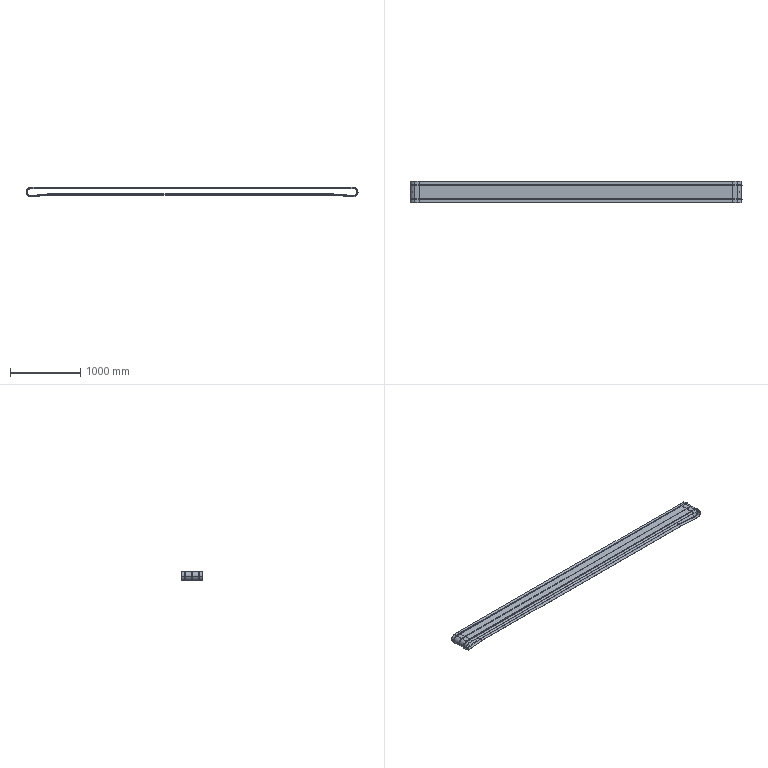Part | STEP file | PVC.BELT.stp | 1 solid | 198 faces | box 4740 x 300 x 138.65 mm | volume 11036267 mm3 | plane 86 | cylinder 64 | cone 48 | commonest cylinder face diameters 58.7 x12 120.3 x12 42.7 x8 64.7 x8 114.3 x8 136.3 x8